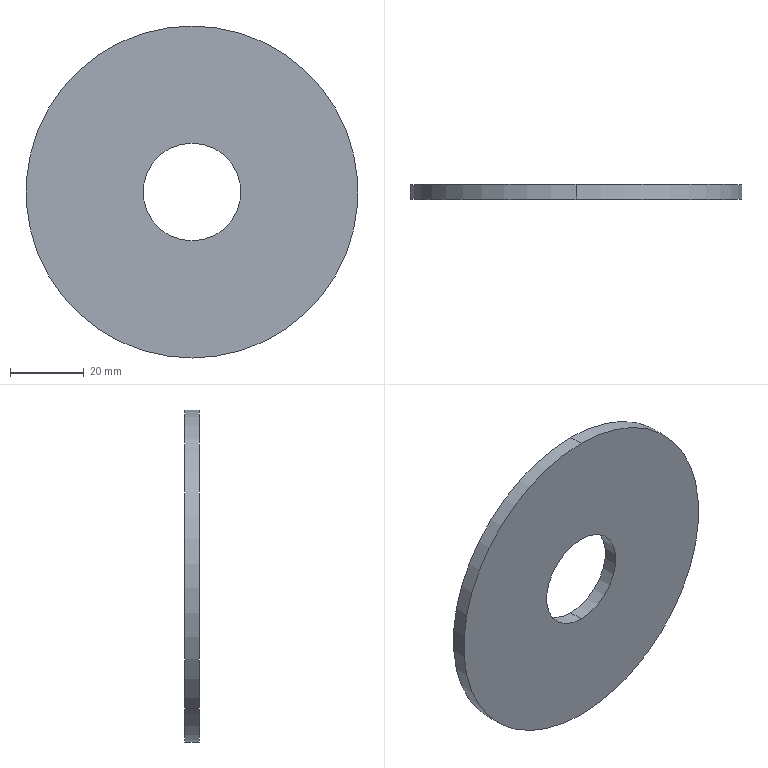Part | SolidWorks | features Extrusion 1, ICE 1 | 1 solid | 6 faces | box 90 x 4 x 90 mm | volume 23241 mm3 | cylinder 4 | plane 2 | commonest cylinder face diameters 26.5 x2 90 x2
STEP:
#1=CARTESIAN_POINT('',(0.,2.,-13.25));
#2=VERTEX_POINT('',#1);
#3=CARTESIAN_POINT('',(0.,2.,13.25));
#4=VERTEX_POINT('',#3);
#5=CARTESIAN_POINT('',(0.,2.,0.));
#6=DIRECTION('',(0.,1.,0.));
#7=DIRECTION('',(0.,0.,1.));
#8=AXIS2_PLACEMENT_3D('',#5,#6,#7);
#9=CIRCLE('',#8,13.25);
#10=EDGE_CURVE('',#2,#4,#9,.T.);
#11=ORIENTED_EDGE('',*,*,#10,.T.);
#12=CARTESIAN_POINT('',(0.,-2.,13.25));
#13=VERTEX_POINT('',#12);
#14=CARTESIAN_POINT('',(0.,2.,13.25));
#15=DIRECTION('',(0.,-1.,0.));
#16=VECTOR('',#15,1000.);
#17=LINE('',#14,#16);
#18=EDGE_CURVE('',#4,#13,#17,.T.);
#19=ORIENTED_EDGE('',*,*,#18,.T.);
#20=CARTESIAN_POINT('',(0.,-2.,-13.25));
#21=VERTEX_POINT('',#20);
#22=CARTESIAN_POINT('',(0.,-2.,0.));
#23=DIRECTION('',(0.,1.,0.));
#24=DIRECTION('',(0.,0.,1.));
#25=AXIS2_PLACEMENT_3D('',#22,#23,#24);
#26=CIRCLE('',#25,13.25);
#27=EDGE_CURVE('',#21,#13,#26,.T.);
#28=ORIENTED_EDGE('',*,*,#27,.F.);
#29=CARTESIAN_POINT('',(0.,2.,-13.25));
#30=DIRECTION('',(0.,-1.,0.));
#31=VECTOR('',#30,1000.);
#32=LINE('',#29,#31);
#33=EDGE_CURVE('',#2,#21,#32,.T.);
#34=ORIENTED_EDGE('',*,*,#33,.F.);
#35=EDGE_LOOP('',(#11,#19,#28,#34));
#36=FACE_OUTER_BOUND('',#35,.T.);
#37=CARTESIAN_POINT('',(0.,2.,0.));
#38=DIRECTION('',(0.,-1.,0.));
#39=DIRECTION('',(0.,0.,-1.));
#40=AXIS2_PLACEMENT_3D('',#37,#38,#39);
#41=CYLINDRICAL_SURFACE('',#40,13.25);
#42=ADVANCED_FACE('',(#36),#41,.F.);
#43=CARTESIAN_POINT('',(0.,2.,45.));
#44=VERTEX_POINT('',#43);
#45=CARTESIAN_POINT('',(0.,2.,-45.));
#46=VERTEX_POINT('',#45);
#47=CARTESIAN_POINT('',(0.,2.,0.));
#48=DIRECTION('',(0.,1.,0.));
#49=DIRECTION('',(0.,0.,1.));
#50=AXIS2_PLACEMENT_3D('',#47,#48,#49);
#51=CIRCLE('',#50,45.);
#52=EDGE_CURVE('',#44,#46,#51,.T.);
#53=ORIENTED_EDGE('',*,*,#52,.F.);
#54=CARTESIAN_POINT('',(0.,-2.,45.));
#55=VERTEX_POINT('',#54);
#56=CARTESIAN_POINT('',(0.,2.,45.));
#57=DIRECTION('',(0.,-1.,0.));
#58=VECTOR('',#57,1000.);
#59=LINE('',#56,#58);
#60=EDGE_CURVE('',#44,#55,#59,.T.);
#61=ORIENTED_EDGE('',*,*,#60,.T.);
#62=CARTESIAN_POINT('',(0.,-2.,-45.));
#63=VERTEX_POINT('',#62);
#64=CARTESIAN_POINT('',(0.,-2.,0.));
#65=DIRECTION('',(0.,1.,0.));
#66=DIRECTION('',(0.,0.,1.));
#67=AXIS2_PLACEMENT_3D('',#64,#65,#66);
#68=CIRCLE('',#67,45.);
#69=EDGE_CURVE('',#55,#63,#68,.T.);
#70=ORIENTED_EDGE('',*,*,#69,.T.);
#71=CARTESIAN_POINT('',(0.,2.,-45.));
#72=DIRECTION('',(0.,-1.,0.));
#73=VECTOR('',#72,1000.);
#74=LINE('',#71,#73);
#75=EDGE_CURVE('',#46,#63,#74,.T.);
#76=ORIENTED_EDGE('',*,*,#75,.F.);
#77=EDGE_LOOP('',(#53,#61,#70,#76));
#78=FACE_OUTER_BOUND('',#77,.T.);
#79=CARTESIAN_POINT('',(0.,2.,0.));
#80=DIRECTION('',(0.,-1.,0.));
#81=DIRECTION('',(0.,0.,-1.));
#82=AXIS2_PLACEMENT_3D('',#79,#80,#81);
#83=CYLINDRICAL_SURFACE('',#82,45.);
#84=ADVANCED_FACE('',(#78),#83,.T.);
#85=CARTESIAN_POINT('',(0.,2.,0.));
#86=DIRECTION('',(0.,1.,0.));
#87=DIRECTION('',(0.,0.,1.));
#88=AXIS2_PLACEMENT_3D('',#85,#86,#87);
#89=CIRCLE('',#88,45.);
#90=EDGE_CURVE('',#46,#44,#89,.T.);
#91=ORIENTED_EDGE('',*,*,#90,.T.);
#92=ORIENTED_EDGE('',*,*,#52,.T.);
#93=EDGE_LOOP('',(#91,#92));
#94=FACE_OUTER_BOUND('',#93,.T.);
#95=ORIENTED_EDGE('',*,*,#10,.F.);
#96=CARTESIAN_POINT('',(0.,2.,0.));
#97=DIRECTION('',(0.,1.,0.));
#98=DIRECTION('',(0.,0.,1.));
#99=AXIS2_PLACEMENT_3D('',#96,#97,#98);
#100=CIRCLE('',#99,13.25);
#101=EDGE_CURVE('',#4,#2,#100,.T.);
#102=ORIENTED_EDGE('',*,*,#101,.F.);
#103=EDGE_LOOP('',(#95,#102));
#104=FACE_BOUND('',#103,.T.);
#105=CARTESIAN_POINT('',(0.,2.,0.));
#106=DIRECTION('',(0.,1.,0.));
#107=DIRECTION('',(0.,0.,1.));
#108=AXIS2_PLACEMENT_3D('',#105,#106,#107);
#109=PLANE('',#108);
#110=ADVANCED_FACE('',(#94,#104),#109,.T.);
#111=CARTESIAN_POINT('',(0.,-2.,0.));
#112=DIRECTION('',(0.,1.,0.));
#113=DIRECTION('',(0.,0.,1.));
#114=AXIS2_PLACEMENT_3D('',#111,#112,#113);
#115=CIRCLE('',#114,45.);
#116=EDGE_CURVE('',#63,#55,#115,.T.);
#117=ORIENTED_EDGE('',*,*,#116,.F.);
#118=ORIENTED_EDGE('',*,*,#69,.F.);
#119=EDGE_LOOP('',(#117,#118));
#120=FACE_OUTER_BOUND('',#119,.T.);
#121=ORIENTED_EDGE('',*,*,#27,.T.);
#122=CARTESIAN_POINT('',(0.,-2.,0.));
#123=DIRECTION('',(0.,1.,0.));
#124=DIRECTION('',(0.,0.,1.));
#125=AXIS2_PLACEMENT_3D('',#122,#123,#124);
#126=CIRCLE('',#125,13.25);
#127=EDGE_CURVE('',#13,#21,#126,.T.);
#128=ORIENTED_EDGE('',*,*,#127,.T.);
#129=EDGE_LOOP('',(#121,#128));
#130=FACE_BOUND('',#129,.T.);
#131=CARTESIAN_POINT('',(0.,-2.,0.));
#132=DIRECTION('',(0.,1.,0.));
#133=DIRECTION('',(0.,0.,1.));
#134=AXIS2_PLACEMENT_3D('',#131,#132,#133);
#135=PLANE('',#134);
#136=ADVANCED_FACE('',(#120,#130),#135,.F.);
#137=ORIENTED_EDGE('',*,*,#60,.F.);
#138=ORIENTED_EDGE('',*,*,#90,.F.);
#139=ORIENTED_EDGE('',*,*,#75,.T.);
#140=ORIENTED_EDGE('',*,*,#116,.T.);
#141=EDGE_LOOP('',(#137,#138,#139,#140));
#142=FACE_OUTER_BOUND('',#141,.T.);
#143=CARTESIAN_POINT('',(0.,2.,0.));
#144=DIRECTION('',(0.,-1.,0.));
#145=DIRECTION('',(0.,0.,-1.));
#146=AXIS2_PLACEMENT_3D('',#143,#144,#145);
#147=CYLINDRICAL_SURFACE('',#146,45.);
#148=ADVANCED_FACE('',(#142),#147,.T.);
#149=ORIENTED_EDGE('',*,*,#18,.F.);
#150=ORIENTED_EDGE('',*,*,#101,.T.);
#151=ORIENTED_EDGE('',*,*,#33,.T.);
#152=ORIENTED_EDGE('',*,*,#127,.F.);
#153=EDGE_LOOP('',(#149,#150,#151,#152));
#154=FACE_OUTER_BOUND('',#153,.T.);
#155=CARTESIAN_POINT('',(0.,2.,0.));
#156=DIRECTION('',(0.,-1.,0.));
#157=DIRECTION('',(0.,0.,-1.));
#158=AXIS2_PLACEMENT_3D('',#155,#156,#157);
#159=CYLINDRICAL_SURFACE('',#158,13.25);
#160=ADVANCED_FACE('',(#154),#159,.F.);
#161=CLOSED_SHELL('',(#42,#84,#110,#136,#148,#160));
#162=MANIFOLD_SOLID_BREP('',#161);
#163=CARTESIAN_POINT('',(0.,0.,0.));
#164=DIRECTION('',(0.,0.,1.));
#165=DIRECTION('',(1.,0.,0.));
#166=AXIS2_PLACEMENT_3D('',#163,#164,#165);
#167=(LENGTH_UNIT()NAMED_UNIT(*)SI_UNIT(.MILLI.,.METRE.));
#168=UNCERTAINTY_MEASURE_WITH_UNIT(LENGTH_MEASURE(0.00001),#167,'','');
#169=(NAMED_UNIT(*)PLANE_ANGLE_UNIT()SI_UNIT($,.RADIAN.));
#170=(NAMED_UNIT(*)SI_UNIT($,.STERADIAN.)SOLID_ANGLE_UNIT());
#171=(GEOMETRIC_REPRESENTATION_CONTEXT(3)GLOBAL_UNCERTAINTY_ASSIGNED_CONTEXT((#168))GLOBAL_UNIT_ASSIGNED_CONTEXT((#167,#169,#170))REPRESENTATION_CONTEXT('',''));
#172=ADVANCED_BREP_SHAPE_REPRESENTATION('',(#162,#166),#171);